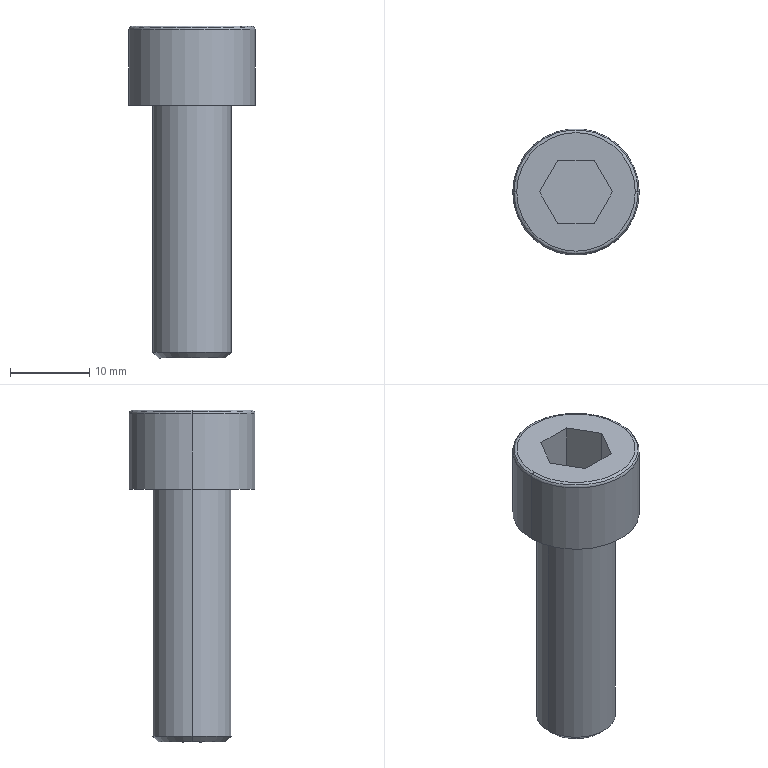Part | Creo | 1 solid | 20 faces | box 16 x 16 x 42 mm | volume 4147 mm3 | plane 10 | cylinder 4 | torus 4 | cone 2 | commonest cylinder face diameters 10 x2 16 x2
STEP:
#1=CARTESIAN_POINT('',(-203.,-159.908,-42.75));
#2=VERTEX_POINT('',#1);
#3=CARTESIAN_POINT('',(-193.,-159.908,-42.75));
#4=VERTEX_POINT('',#3);
#5=CARTESIAN_POINT('',(-198.,-159.908,-42.75));
#6=DIRECTION('',(0.,0.,-1.));
#7=DIRECTION('',(-1.,0.,0.));
#8=AXIS2_PLACEMENT_3D('',#5,#6,#7);
#9=CIRCLE('',#8,5.);
#10=EDGE_CURVE('',#2,#4,#9,.T.);
#11=ORIENTED_EDGE('',*,*,#10,.T.);
#12=CARTESIAN_POINT('',(-193.,-159.908,-11.5));
#13=VERTEX_POINT('',#12);
#14=CARTESIAN_POINT('',(-193.,-159.908,-42.75));
#15=DIRECTION('',(0.,0.,1.));
#16=VECTOR('',#15,31.25);
#17=LINE('',#14,#16);
#18=EDGE_CURVE('',#4,#13,#17,.T.);
#19=ORIENTED_EDGE('',*,*,#18,.T.);
#20=CARTESIAN_POINT('',(-203.,-159.908,-11.5));
#21=VERTEX_POINT('',#20);
#22=CARTESIAN_POINT('',(-198.,-159.908,-11.5));
#23=DIRECTION('',(0.,0.,1.));
#24=DIRECTION('',(1.,0.,0.));
#25=AXIS2_PLACEMENT_3D('',#22,#23,#24);
#26=CIRCLE('',#25,5.);
#27=EDGE_CURVE('',#13,#21,#26,.T.);
#28=ORIENTED_EDGE('',*,*,#27,.T.);
#29=CARTESIAN_POINT('',(-203.,-159.908,-42.75));
#30=DIRECTION('',(0.,0.,1.));
#31=VECTOR('',#30,31.25);
#32=LINE('',#29,#31);
#33=EDGE_CURVE('',#2,#21,#32,.T.);
#34=ORIENTED_EDGE('',*,*,#33,.F.);
#35=EDGE_LOOP('',(#11,#19,#28,#34));
#36=FACE_OUTER_BOUND('',#35,.F.);
#37=CARTESIAN_POINT('',(-198.,-159.908,-43.5));
#38=DIRECTION('',(0.,0.,1.));
#39=DIRECTION('',(1.,0.,0.));
#40=AXIS2_PLACEMENT_3D('',#37,#38,#39);
#41=CYLINDRICAL_SURFACE('',#40,5.);
#42=ADVANCED_FACE('',(#36),#41,.T.);
#43=CARTESIAN_POINT('',(-202.25,-159.908,-43.5));
#44=VERTEX_POINT('',#43);
#45=CARTESIAN_POINT('',(-193.75,-159.908,-43.5));
#46=VERTEX_POINT('',#45);
#47=CARTESIAN_POINT('',(-198.,-159.908,-43.5));
#48=DIRECTION('',(0.,0.,-1.));
#49=DIRECTION('',(-1.,0.,0.));
#50=AXIS2_PLACEMENT_3D('',#47,#48,#49);
#51=CIRCLE('',#50,4.25);
#52=EDGE_CURVE('',#44,#46,#51,.T.);
#53=ORIENTED_EDGE('',*,*,#52,.T.);
#54=CARTESIAN_POINT('',(-193.75,-159.908,-43.5));
#55=DIRECTION('',(0.7071,0.,0.7071));
#56=VECTOR('',#55,1.061);
#57=LINE('',#54,#56);
#58=EDGE_CURVE('',#46,#4,#57,.T.);
#59=ORIENTED_EDGE('',*,*,#58,.T.);
#60=ORIENTED_EDGE('',*,*,#10,.F.);
#61=CARTESIAN_POINT('',(-202.25,-159.908,-43.5));
#62=DIRECTION('',(-0.7071,0.,0.7071));
#63=VECTOR('',#62,1.061);
#64=LINE('',#61,#63);
#65=EDGE_CURVE('',#44,#2,#64,.T.);
#66=ORIENTED_EDGE('',*,*,#65,.F.);
#67=EDGE_LOOP('',(#53,#59,#60,#66));
#68=FACE_OUTER_BOUND('',#67,.F.);
#69=CARTESIAN_POINT('',(-198.,-159.908,-43.125));
#70=DIRECTION('',(0.,0.,1.));
#71=DIRECTION('',(1.,0.,0.));
#72=AXIS2_PLACEMENT_3D('',#69,#70,#71);
#73=CONICAL_SURFACE('',#72,4.625,45.);
#74=ADVANCED_FACE('',(#68),#73,.T.);
#75=CARTESIAN_POINT('',(-198.,-159.908,-43.5));
#76=DIRECTION('',(0.,0.,-1.));
#77=DIRECTION('',(1.,0.,0.));
#78=AXIS2_PLACEMENT_3D('',#75,#76,#77);
#79=CIRCLE('',#78,4.25);
#80=EDGE_CURVE('',#46,#44,#79,.T.);
#81=ORIENTED_EDGE('',*,*,#80,.F.);
#82=ORIENTED_EDGE('',*,*,#52,.F.);
#83=EDGE_LOOP('',(#81,#82));
#84=FACE_OUTER_BOUND('',#83,.F.);
#85=CARTESIAN_POINT('',(-198.,-159.908,-43.5));
#86=DIRECTION('',(0.,0.,1.));
#87=DIRECTION('',(1.,0.,0.));
#88=AXIS2_PLACEMENT_3D('',#85,#86,#87);
#89=PLANE('',#88);
#90=ADVANCED_FACE('',(#84),#89,.F.);
#91=ORIENTED_EDGE('',*,*,#80,.T.);
#92=ORIENTED_EDGE('',*,*,#65,.T.);
#93=CARTESIAN_POINT('',(-198.,-159.908,-42.75));
#94=DIRECTION('',(0.,0.,-1.));
#95=DIRECTION('',(1.,0.,0.));
#96=AXIS2_PLACEMENT_3D('',#93,#94,#95);
#97=CIRCLE('',#96,5.);
#98=EDGE_CURVE('',#4,#2,#97,.T.);
#99=ORIENTED_EDGE('',*,*,#98,.F.);
#100=ORIENTED_EDGE('',*,*,#58,.F.);
#101=EDGE_LOOP('',(#91,#92,#99,#100));
#102=FACE_OUTER_BOUND('',#101,.F.);
#103=CARTESIAN_POINT('',(-198.,-159.908,-43.125));
#104=DIRECTION('',(0.,0.,1.));
#105=DIRECTION('',(1.,0.,0.));
#106=AXIS2_PLACEMENT_3D('',#103,#104,#105);
#107=CONICAL_SURFACE('',#106,4.625,45.);
#108=ADVANCED_FACE('',(#102),#107,.T.);
#109=ORIENTED_EDGE('',*,*,#98,.T.);
#110=ORIENTED_EDGE('',*,*,#33,.T.);
#111=CARTESIAN_POINT('',(-198.,-159.908,-11.5));
#112=DIRECTION('',(0.,0.,1.));
#113=DIRECTION('',(-1.,0.,0.));
#114=AXIS2_PLACEMENT_3D('',#111,#112,#113);
#115=CIRCLE('',#114,5.);
#116=EDGE_CURVE('',#21,#13,#115,.T.);
#117=ORIENTED_EDGE('',*,*,#116,.T.);
#118=ORIENTED_EDGE('',*,*,#18,.F.);
#119=EDGE_LOOP('',(#109,#110,#117,#118));
#120=FACE_OUTER_BOUND('',#119,.F.);
#121=CARTESIAN_POINT('',(-198.,-159.908,-43.5));
#122=DIRECTION('',(0.,0.,1.));
#123=DIRECTION('',(1.,0.,0.));
#124=AXIS2_PLACEMENT_3D('',#121,#122,#123);
#125=CYLINDRICAL_SURFACE('',#124,5.);
#126=ADVANCED_FACE('',(#120),#125,.T.);
#127=CARTESIAN_POINT('',(-190.,-159.908,-11.5));
#128=VERTEX_POINT('',#127);
#129=CARTESIAN_POINT('',(-206.,-159.908,-11.5));
#130=VERTEX_POINT('',#129);
#131=CARTESIAN_POINT('',(-198.,-159.908,-11.5));
#132=DIRECTION('',(0.,0.,-1.));
#133=DIRECTION('',(1.,0.,0.));
#134=AXIS2_PLACEMENT_3D('',#131,#132,#133);
#135=CIRCLE('',#134,8.);
#136=EDGE_CURVE('',#128,#130,#135,.T.);
#137=ORIENTED_EDGE('',*,*,#136,.F.);
#138=CARTESIAN_POINT('',(-198.,-159.908,-11.5));
#139=DIRECTION('',(0.,0.,-1.));
#140=DIRECTION('',(-1.,0.,0.));
#141=AXIS2_PLACEMENT_3D('',#138,#139,#140);
#142=CIRCLE('',#141,8.);
#143=EDGE_CURVE('',#130,#128,#142,.T.);
#144=ORIENTED_EDGE('',*,*,#143,.F.);
#145=EDGE_LOOP('',(#137,#144));
#146=FACE_OUTER_BOUND('',#145,.F.);
#147=ORIENTED_EDGE('',*,*,#27,.F.);
#148=ORIENTED_EDGE('',*,*,#116,.F.);
#149=EDGE_LOOP('',(#147,#148));
#150=FACE_BOUND('',#149,.F.);
#151=CARTESIAN_POINT('',(-198.,-159.908,-11.5));
#152=DIRECTION('',(0.,0.,-1.));
#153=DIRECTION('',(-1.,0.,0.));
#154=AXIS2_PLACEMENT_3D('',#151,#152,#153);
#155=PLANE('',#154);
#156=ADVANCED_FACE('',(#146,#150),#155,.T.);
#157=CARTESIAN_POINT('',(-206.,-159.908,-2.));
#158=VERTEX_POINT('',#157);
#159=CARTESIAN_POINT('',(-190.,-159.908,-2.));
#160=VERTEX_POINT('',#159);
#161=CARTESIAN_POINT('',(-198.,-159.908,-2.));
#162=DIRECTION('',(0.,0.,1.));
#163=DIRECTION('',(-1.,0.,0.));
#164=AXIS2_PLACEMENT_3D('',#161,#162,#163);
#165=CIRCLE('',#164,8.);
#166=EDGE_CURVE('',#158,#160,#165,.T.);
#167=ORIENTED_EDGE('',*,*,#166,.T.);
#168=CARTESIAN_POINT('',(-190.,-159.908,-11.5));
#169=DIRECTION('',(0.,0.,1.));
#170=VECTOR('',#169,9.5);
#171=LINE('',#168,#170);
#172=EDGE_CURVE('',#128,#160,#171,.T.);
#173=ORIENTED_EDGE('',*,*,#172,.F.);
#174=ORIENTED_EDGE('',*,*,#136,.T.);
#175=CARTESIAN_POINT('',(-206.,-159.908,-11.5));
#176=DIRECTION('',(0.,0.,1.));
#177=VECTOR('',#176,9.5);
#178=LINE('',#175,#177);
#179=EDGE_CURVE('',#130,#158,#178,.T.);
#180=ORIENTED_EDGE('',*,*,#179,.T.);
#181=EDGE_LOOP('',(#167,#173,#174,#180));
#182=FACE_OUTER_BOUND('',#181,.F.);
#183=CARTESIAN_POINT('',(-198.,-159.908,-11.5));
#184=DIRECTION('',(0.,0.,1.));
#185=DIRECTION('',(1.,0.,0.));
#186=AXIS2_PLACEMENT_3D('',#183,#184,#185);
#187=CYLINDRICAL_SURFACE('',#186,8.);
#188=ADVANCED_FACE('',(#182),#187,.T.);
#189=ORIENTED_EDGE('',*,*,#166,.F.);
#190=CARTESIAN_POINT('',(-205.854,-159.908,-1.646));
#191=VERTEX_POINT('',#190);
#192=CARTESIAN_POINT('',(-205.5,-159.908,-2.));
#193=DIRECTION('',(0.,1.,0.));
#194=DIRECTION('',(-1.,0.,0.));
#195=AXIS2_PLACEMENT_3D('',#192,#193,#194);
#196=CIRCLE('',#195,0.5);
#197=EDGE_CURVE('',#158,#191,#196,.T.);
#198=ORIENTED_EDGE('',*,*,#197,.T.);
#199=CARTESIAN_POINT('',(-190.146,-159.908,-1.646));
#200=VERTEX_POINT('',#199);
#201=CARTESIAN_POINT('',(-198.,-159.908,-1.646));
#202=DIRECTION('',(0.,0.,1.));
#203=DIRECTION('',(-1.,0.,0.));
#204=AXIS2_PLACEMENT_3D('',#201,#202,#203);
#205=CIRCLE('',#204,7.854);
#206=EDGE_CURVE('',#191,#200,#205,.T.);
#207=ORIENTED_EDGE('',*,*,#206,.T.);
#208=CARTESIAN_POINT('',(-190.5,-159.908,-2.));
#209=DIRECTION('',(0.,-1.,0.));
#210=DIRECTION('',(1.,0.,0.));
#211=AXIS2_PLACEMENT_3D('',#208,#209,#210);
#212=CIRCLE('',#211,0.5);
#213=EDGE_CURVE('',#160,#200,#212,.T.);
#214=ORIENTED_EDGE('',*,*,#213,.F.);
#215=EDGE_LOOP('',(#189,#198,#207,#214));
#216=FACE_OUTER_BOUND('',#215,.F.);
#217=CARTESIAN_POINT('',(-198.,-159.908,-2.));
#218=DIRECTION('',(0.,0.,1.));
#219=DIRECTION('',(1.,0.,0.));
#220=AXIS2_PLACEMENT_3D('',#217,#218,#219);
#221=TOROIDAL_SURFACE('',#220,7.5,0.5);
#222=ADVANCED_FACE('',(#216),#221,.T.);
#223=CARTESIAN_POINT('',(-198.,-159.908,-2.));
#224=DIRECTION('',(0.,0.,1.));
#225=DIRECTION('',(1.,0.,0.));
#226=AXIS2_PLACEMENT_3D('',#223,#224,#225);
#227=CIRCLE('',#226,8.);
#228=EDGE_CURVE('',#160,#158,#227,.T.);
#229=ORIENTED_EDGE('',*,*,#228,.F.);
#230=ORIENTED_EDGE('',*,*,#213,.T.);
#231=CARTESIAN_POINT('',(-198.,-159.908,-1.646));
#232=DIRECTION('',(0.,0.,1.));
#233=DIRECTION('',(1.,0.,0.));
#234=AXIS2_PLACEMENT_3D('',#231,#232,#233);
#235=CIRCLE('',#234,7.854);
#236=EDGE_CURVE('',#200,#191,#235,.T.);
#237=ORIENTED_EDGE('',*,*,#236,.T.);
#238=ORIENTED_EDGE('',*,*,#197,.F.);
#239=EDGE_LOOP('',(#229,#230,#237,#238));
#240=FACE_OUTER_BOUND('',#239,.F.);
#241=CARTESIAN_POINT('',(-198.,-159.908,-2.));
#242=DIRECTION('',(0.,0.,1.));
#243=DIRECTION('',(1.,0.,0.));
#244=AXIS2_PLACEMENT_3D('',#241,#242,#243);
#245=TOROIDAL_SURFACE('',#244,7.5,0.5);
#246=ADVANCED_FACE('',(#240),#245,.T.);
#247=ORIENTED_EDGE('',*,*,#228,.T.);
#248=ORIENTED_EDGE('',*,*,#179,.F.);
#249=ORIENTED_EDGE('',*,*,#143,.T.);
#250=ORIENTED_EDGE('',*,*,#172,.T.);
#251=EDGE_LOOP('',(#247,#248,#249,#250));
#252=FACE_OUTER_BOUND('',#251,.F.);
#253=CARTESIAN_POINT('',(-198.,-159.908,-11.5));
#254=DIRECTION('',(0.,0.,1.));
#255=DIRECTION('',(1.,0.,0.));
#256=AXIS2_PLACEMENT_3D('',#253,#254,#255);
#257=CYLINDRICAL_SURFACE('',#256,8.);
#258=ADVANCED_FACE('',(#252),#257,.T.);
#259=CARTESIAN_POINT('',(-190.5,-159.908,-1.5));
#260=VERTEX_POINT('',#259);
#261=CARTESIAN_POINT('',(-205.5,-159.908,-1.5));
#262=VERTEX_POINT('',#261);
#263=CARTESIAN_POINT('',(-198.,-159.908,-1.5));
#264=DIRECTION('',(0.,0.,1.));
#265=DIRECTION('',(1.,0.,0.));
#266=AXIS2_PLACEMENT_3D('',#263,#264,#265);
#267=CIRCLE('',#266,7.5);
#268=EDGE_CURVE('',#260,#262,#267,.T.);
#269=ORIENTED_EDGE('',*,*,#268,.T.);
#270=CARTESIAN_POINT('',(-205.5,-159.908,-2.));
#271=DIRECTION('',(0.,1.,0.));
#272=DIRECTION('',(-0.7071,0.,0.7071));
#273=AXIS2_PLACEMENT_3D('',#270,#271,#272);
#274=CIRCLE('',#273,0.5);
#275=EDGE_CURVE('',#191,#262,#274,.T.);
#276=ORIENTED_EDGE('',*,*,#275,.F.);
#277=ORIENTED_EDGE('',*,*,#236,.F.);
#278=CARTESIAN_POINT('',(-190.5,-159.908,-2.));
#279=DIRECTION('',(0.,-1.,0.));
#280=DIRECTION('',(0.7071,0.,0.7071));
#281=AXIS2_PLACEMENT_3D('',#278,#279,#280);
#282=CIRCLE('',#281,0.5);
#283=EDGE_CURVE('',#200,#260,#282,.T.);
#284=ORIENTED_EDGE('',*,*,#283,.T.);
#285=EDGE_LOOP('',(#269,#276,#277,#284));
#286=FACE_OUTER_BOUND('',#285,.F.);
#287=CARTESIAN_POINT('',(-198.,-159.908,-2.));
#288=DIRECTION('',(0.,0.,1.));
#289=DIRECTION('',(1.,0.,0.));
#290=AXIS2_PLACEMENT_3D('',#287,#288,#289);
#291=TOROIDAL_SURFACE('',#290,7.5,0.5);
#292=ADVANCED_FACE('',(#286),#291,.T.);
#293=ORIENTED_EDGE('',*,*,#268,.F.);
#294=CARTESIAN_POINT('',(-198.,-159.908,-1.5));
#295=DIRECTION('',(0.,0.,1.));
#296=DIRECTION('',(-1.,0.,0.));
#297=AXIS2_PLACEMENT_3D('',#294,#295,#296);
#298=CIRCLE('',#297,7.5);
#299=EDGE_CURVE('',#262,#260,#298,.T.);
#300=ORIENTED_EDGE('',*,*,#299,.F.);
#301=EDGE_LOOP('',(#293,#300));
#302=FACE_OUTER_BOUND('',#301,.F.);
#303=CARTESIAN_POINT('',(-195.691,-155.908,-1.5));
#304=VERTEX_POINT('',#303);
#305=CARTESIAN_POINT('',(-200.309,-155.908,-1.5));
#306=VERTEX_POINT('',#305);
#307=CARTESIAN_POINT('',(-195.691,-155.908,-1.5));
#308=DIRECTION('',(-1.,0.,0.));
#309=VECTOR('',#308,4.619);
#310=LINE('',#307,#309);
#311=EDGE_CURVE('',#304,#306,#310,.T.);
#312=ORIENTED_EDGE('',*,*,#311,.T.);
#313=CARTESIAN_POINT('',(-202.619,-159.908,-1.5));
#314=VERTEX_POINT('',#313);
#315=CARTESIAN_POINT('',(-202.619,-159.908,-1.5));
#316=DIRECTION('',(0.5,0.866,0.));
#317=VECTOR('',#316,4.619);
#318=LINE('',#315,#317);
#319=EDGE_CURVE('',#314,#306,#318,.T.);
#320=ORIENTED_EDGE('',*,*,#319,.F.);
#321=CARTESIAN_POINT('',(-200.309,-163.908,-1.5));
#322=VERTEX_POINT('',#321);
#323=CARTESIAN_POINT('',(-200.309,-163.908,-1.5));
#324=DIRECTION('',(-0.5,0.866,0.));
#325=VECTOR('',#324,4.619);
#326=LINE('',#323,#325);
#327=EDGE_CURVE('',#322,#314,#326,.T.);
#328=ORIENTED_EDGE('',*,*,#327,.F.);
#329=CARTESIAN_POINT('',(-195.691,-163.908,-1.5));
#330=VERTEX_POINT('',#329);
#331=CARTESIAN_POINT('',(-200.309,-163.908,-1.5));
#332=DIRECTION('',(1.,0.,0.));
#333=VECTOR('',#332,4.619);
#334=LINE('',#331,#333);
#335=EDGE_CURVE('',#322,#330,#334,.T.);
#336=ORIENTED_EDGE('',*,*,#335,.T.);
#337=CARTESIAN_POINT('',(-193.381,-159.908,-1.5));
#338=VERTEX_POINT('',#337);
#339=CARTESIAN_POINT('',(-193.381,-159.908,-1.5));
#340=DIRECTION('',(-0.5,-0.866,0.));
#341=VECTOR('',#340,4.619);
#342=LINE('',#339,#341);
#343=EDGE_CURVE('',#338,#330,#342,.T.);
#344=ORIENTED_EDGE('',*,*,#343,.F.);
#345=CARTESIAN_POINT('',(-195.691,-155.908,-1.5));
#346=DIRECTION('',(0.5,-0.866,0.));
#347=VECTOR('',#346,4.619);
#348=LINE('',#345,#347);
#349=EDGE_CURVE('',#304,#338,#348,.T.);
#350=ORIENTED_EDGE('',*,*,#349,.F.);
#351=EDGE_LOOP('',(#312,#320,#328,#336,#344,#350));
#352=FACE_BOUND('',#351,.F.);
#353=CARTESIAN_POINT('',(-198.,-159.908,-1.5));
#354=DIRECTION('',(0.,0.,1.));
#355=DIRECTION('',(1.,0.,0.));
#356=AXIS2_PLACEMENT_3D('',#353,#354,#355);
#357=PLANE('',#356);
#358=ADVANCED_FACE('',(#302,#352),#357,.T.);
#359=ORIENTED_EDGE('',*,*,#299,.T.);
#360=ORIENTED_EDGE('',*,*,#283,.F.);
#361=ORIENTED_EDGE('',*,*,#206,.F.);
#362=ORIENTED_EDGE('',*,*,#275,.T.);
#363=EDGE_LOOP('',(#359,#360,#361,#362));
#364=FACE_OUTER_BOUND('',#363,.F.);
#365=CARTESIAN_POINT('',(-198.,-159.908,-2.));
#366=DIRECTION('',(0.,0.,1.));
#367=DIRECTION('',(1.,0.,0.));
#368=AXIS2_PLACEMENT_3D('',#365,#366,#367);
#369=TOROIDAL_SURFACE('',#368,7.5,0.5);
#370=ADVANCED_FACE('',(#364),#369,.T.);
#371=ORIENTED_EDGE('',*,*,#311,.F.);
#372=CARTESIAN_POINT('',(-195.691,-155.908,-8.1));
#373=VERTEX_POINT('',#372);
#374=CARTESIAN_POINT('',(-195.691,-155.908,-1.5));
#375=DIRECTION('',(0.,0.,-1.));
#376=VECTOR('',#375,6.6);
#377=LINE('',#374,#376);
#378=EDGE_CURVE('',#304,#373,#377,.T.);
#379=ORIENTED_EDGE('',*,*,#378,.T.);
#380=CARTESIAN_POINT('',(-200.309,-155.908,-8.1));
#381=VERTEX_POINT('',#380);
#382=CARTESIAN_POINT('',(-195.691,-155.908,-8.1));
#383=DIRECTION('',(-1.,0.,0.));
#384=VECTOR('',#383,4.619);
#385=LINE('',#382,#384);
#386=EDGE_CURVE('',#373,#381,#385,.T.);
#387=ORIENTED_EDGE('',*,*,#386,.T.);
#388=CARTESIAN_POINT('',(-200.309,-155.908,-1.5));
#389=DIRECTION('',(0.,0.,-1.));
#390=VECTOR('',#389,6.6);
#391=LINE('',#388,#390);
#392=EDGE_CURVE('',#306,#381,#391,.T.);
#393=ORIENTED_EDGE('',*,*,#392,.F.);
#394=EDGE_LOOP('',(#371,#379,#387,#393));
#395=FACE_OUTER_BOUND('',#394,.F.);
#396=CARTESIAN_POINT('',(-200.309,-155.908,-8.1));
#397=DIRECTION('',(0.,1.,0.));
#398=DIRECTION('',(0.,0.,-1.));
#399=AXIS2_PLACEMENT_3D('',#396,#397,#398);
#400=PLANE('',#399);
#401=ADVANCED_FACE('',(#395),#400,.F.);
#402=ORIENTED_EDGE('',*,*,#349,.T.);
#403=CARTESIAN_POINT('',(-193.381,-159.908,-8.1));
#404=VERTEX_POINT('',#403);
#405=CARTESIAN_POINT('',(-193.381,-159.908,-1.5));
#406=DIRECTION('',(0.,0.,-1.));
#407=VECTOR('',#406,6.6);
#408=LINE('',#405,#407);
#409=EDGE_CURVE('',#338,#404,#408,.T.);
#410=ORIENTED_EDGE('',*,*,#409,.T.);
#411=CARTESIAN_POINT('',(-193.381,-159.908,-8.1));
#412=DIRECTION('',(-0.5,0.866,0.));
#413=VECTOR('',#412,4.619);
#414=LINE('',#411,#413);
#415=EDGE_CURVE('',#404,#373,#414,.T.);
#416=ORIENTED_EDGE('',*,*,#415,.T.);
#417=ORIENTED_EDGE('',*,*,#378,.F.);
#418=EDGE_LOOP('',(#402,#410,#416,#417));
#419=FACE_OUTER_BOUND('',#418,.F.);
#420=CARTESIAN_POINT('',(-195.691,-155.908,-8.1));
#421=DIRECTION('',(0.866,0.5,0.));
#422=DIRECTION('',(0.5,-0.866,0.));
#423=AXIS2_PLACEMENT_3D('',#420,#421,#422);
#424=PLANE('',#423);
#425=ADVANCED_FACE('',(#419),#424,.F.);
#426=ORIENTED_EDGE('',*,*,#343,.T.);
#427=CARTESIAN_POINT('',(-195.691,-163.908,-8.1));
#428=VERTEX_POINT('',#427);
#429=CARTESIAN_POINT('',(-195.691,-163.908,-1.5));
#430=DIRECTION('',(0.,0.,-1.));
#431=VECTOR('',#430,6.6);
#432=LINE('',#429,#431);
#433=EDGE_CURVE('',#330,#428,#432,.T.);
#434=ORIENTED_EDGE('',*,*,#433,.T.);
#435=CARTESIAN_POINT('',(-195.691,-163.908,-8.1));
#436=DIRECTION('',(0.5,0.866,0.));
#437=VECTOR('',#436,4.619);
#438=LINE('',#435,#437);
#439=EDGE_CURVE('',#428,#404,#438,.T.);
#440=ORIENTED_EDGE('',*,*,#439,.T.);
#441=ORIENTED_EDGE('',*,*,#409,.F.);
#442=EDGE_LOOP('',(#426,#434,#440,#441));
#443=FACE_OUTER_BOUND('',#442,.F.);
#444=CARTESIAN_POINT('',(-193.381,-159.908,-8.1));
#445=DIRECTION('',(0.866,-0.5,0.));
#446=DIRECTION('',(-0.5,-0.866,0.));
#447=AXIS2_PLACEMENT_3D('',#444,#445,#446);
#448=PLANE('',#447);
#449=ADVANCED_FACE('',(#443),#448,.F.);
#450=ORIENTED_EDGE('',*,*,#335,.F.);
#451=CARTESIAN_POINT('',(-200.309,-163.908,-8.1));
#452=VERTEX_POINT('',#451);
#453=CARTESIAN_POINT('',(-200.309,-163.908,-1.5));
#454=DIRECTION('',(0.,0.,-1.));
#455=VECTOR('',#454,6.6);
#456=LINE('',#453,#455);
#457=EDGE_CURVE('',#322,#452,#456,.T.);
#458=ORIENTED_EDGE('',*,*,#457,.T.);
#459=CARTESIAN_POINT('',(-200.309,-163.908,-8.1));
#460=DIRECTION('',(1.,0.,0.));
#461=VECTOR('',#460,4.619);
#462=LINE('',#459,#461);
#463=EDGE_CURVE('',#452,#428,#462,.T.);
#464=ORIENTED_EDGE('',*,*,#463,.T.);
#465=ORIENTED_EDGE('',*,*,#433,.F.);
#466=EDGE_LOOP('',(#450,#458,#464,#465));
#467=FACE_OUTER_BOUND('',#466,.F.);
#468=CARTESIAN_POINT('',(-195.691,-163.908,-8.1));
#469=DIRECTION('',(0.,-1.,0.));
#470=DIRECTION('',(0.,0.,1.));
#471=AXIS2_PLACEMENT_3D('',#468,#469,#470);
#472=PLANE('',#471);
#473=ADVANCED_FACE('',(#467),#472,.F.);
#474=ORIENTED_EDGE('',*,*,#327,.T.);
#475=CARTESIAN_POINT('',(-202.619,-159.908,-8.1));
#476=VERTEX_POINT('',#475);
#477=CARTESIAN_POINT('',(-202.619,-159.908,-1.5));
#478=DIRECTION('',(0.,0.,-1.));
#479=VECTOR('',#478,6.6);
#480=LINE('',#477,#479);
#481=EDGE_CURVE('',#314,#476,#480,.T.);
#482=ORIENTED_EDGE('',*,*,#481,.T.);
#483=CARTESIAN_POINT('',(-202.619,-159.908,-8.1));
#484=DIRECTION('',(0.5,-0.866,0.));
#485=VECTOR('',#484,4.619);
#486=LINE('',#483,#485);
#487=EDGE_CURVE('',#476,#452,#486,.T.);
#488=ORIENTED_EDGE('',*,*,#487,.T.);
#489=ORIENTED_EDGE('',*,*,#457,.F.);
#490=EDGE_LOOP('',(#474,#482,#488,#489));
#491=FACE_OUTER_BOUND('',#490,.F.);
#492=CARTESIAN_POINT('',(-200.309,-163.908,-8.1));
#493=DIRECTION('',(-0.866,-0.5,0.));
#494=DIRECTION('',(-0.5,0.866,0.));
#495=AXIS2_PLACEMENT_3D('',#492,#493,#494);
#496=PLANE('',#495);
#497=ADVANCED_FACE('',(#491),#496,.F.);
#498=ORIENTED_EDGE('',*,*,#319,.T.);
#499=ORIENTED_EDGE('',*,*,#392,.T.);
#500=CARTESIAN_POINT('',(-200.309,-155.908,-8.1));
#501=DIRECTION('',(-0.5,-0.866,0.));
#502=VECTOR('',#501,4.619);
#503=LINE('',#500,#502);
#504=EDGE_CURVE('',#381,#476,#503,.T.);
#505=ORIENTED_EDGE('',*,*,#504,.T.);
#506=ORIENTED_EDGE('',*,*,#481,.F.);
#507=EDGE_LOOP('',(#498,#499,#505,#506));
#508=FACE_OUTER_BOUND('',#507,.F.);
#509=CARTESIAN_POINT('',(-202.619,-159.908,-8.1));
#510=DIRECTION('',(-0.866,0.5,0.));
#511=DIRECTION('',(0.5,0.866,0.));
#512=AXIS2_PLACEMENT_3D('',#509,#510,#511);
#513=PLANE('',#512);
#514=ADVANCED_FACE('',(#508),#513,.F.);
#515=ORIENTED_EDGE('',*,*,#386,.F.);
#516=ORIENTED_EDGE('',*,*,#415,.F.);
#517=ORIENTED_EDGE('',*,*,#439,.F.);
#518=ORIENTED_EDGE('',*,*,#463,.F.);
#519=ORIENTED_EDGE('',*,*,#487,.F.);
#520=ORIENTED_EDGE('',*,*,#504,.F.);
#521=EDGE_LOOP('',(#515,#516,#517,#518,#519,#520));
#522=FACE_OUTER_BOUND('',#521,.F.);
#523=CARTESIAN_POINT('',(-195.691,-155.908,-8.1));
#524=DIRECTION('',(0.,0.,1.));
#525=DIRECTION('',(1.,0.,0.));
#526=AXIS2_PLACEMENT_3D('',#523,#524,#525);
#527=PLANE('',#526);
#528=ADVANCED_FACE('',(#522),#527,.T.);
#529=CLOSED_SHELL('',(#42,#74,#90,#108,#126,#156,#188,#222,#246,#258,#292,#358,#370,#401,#425,#449,#473,#497,#514,#528));
#530=MANIFOLD_SOLID_BREP('',#529);
#531=(LENGTH_UNIT()NAMED_UNIT(*)SI_UNIT(.MILLI.,.METRE.));
#532=UNCERTAINTY_MEASURE_WITH_UNIT(LENGTH_MEASURE(0.004771),#531,'','');
#533=(NAMED_UNIT(*)PLANE_ANGLE_UNIT()SI_UNIT($,.RADIAN.));
#534=PLANE_ANGLE_MEASURE_WITH_UNIT(PLANE_ANGLE_MEASURE(0.01745),#533);
#535=(CONVERSION_BASED_UNIT('DEGREE',#534)NAMED_UNIT(*)PLANE_ANGLE_UNIT());
#536=(NAMED_UNIT(*)SI_UNIT($,.STERADIAN.)SOLID_ANGLE_UNIT());
#537=(GEOMETRIC_REPRESENTATION_CONTEXT(3)GLOBAL_UNCERTAINTY_ASSIGNED_CONTEXT((#532))GLOBAL_UNIT_ASSIGNED_CONTEXT((#531,#535,#536))REPRESENTATION_CONTEXT('',''));
#538=ADVANCED_BREP_SHAPE_REPRESENTATION('',(#530),#537);